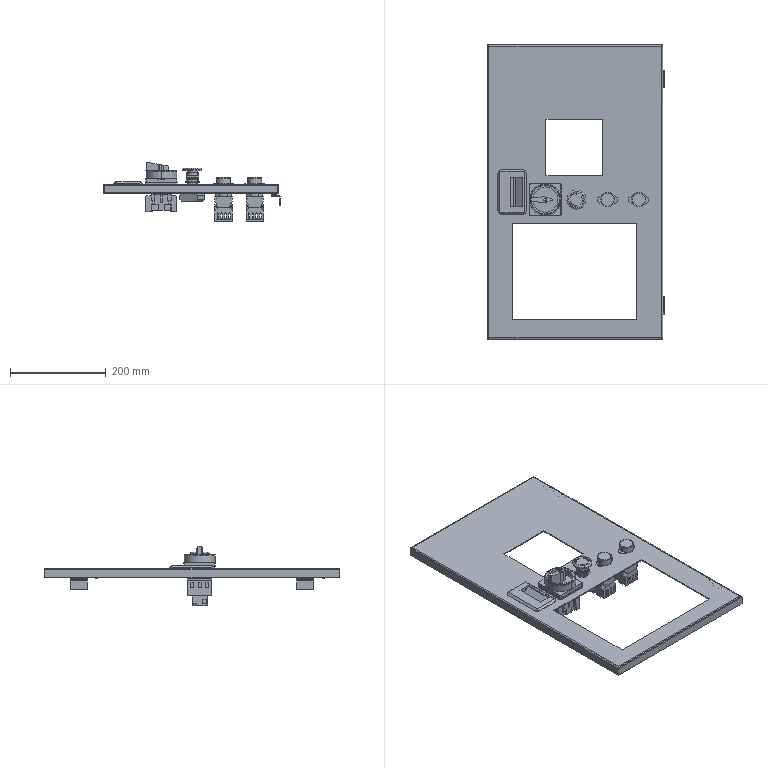Part | SolidWorks | features ReferencePattern 3, CompositeCurve 1, LocalLPattern 1 | 10 solids | 1796 faces | box 369.222 x 614 x 123.704 mm | volume 919283 mm3 | plane 1301 | cylinder 311 | spline 142 | torus 34 | cone 8 | commonest cylinder face diameters 26 x51 4 x36 4.5 x28 2.937 x24 5 x20 30 x16